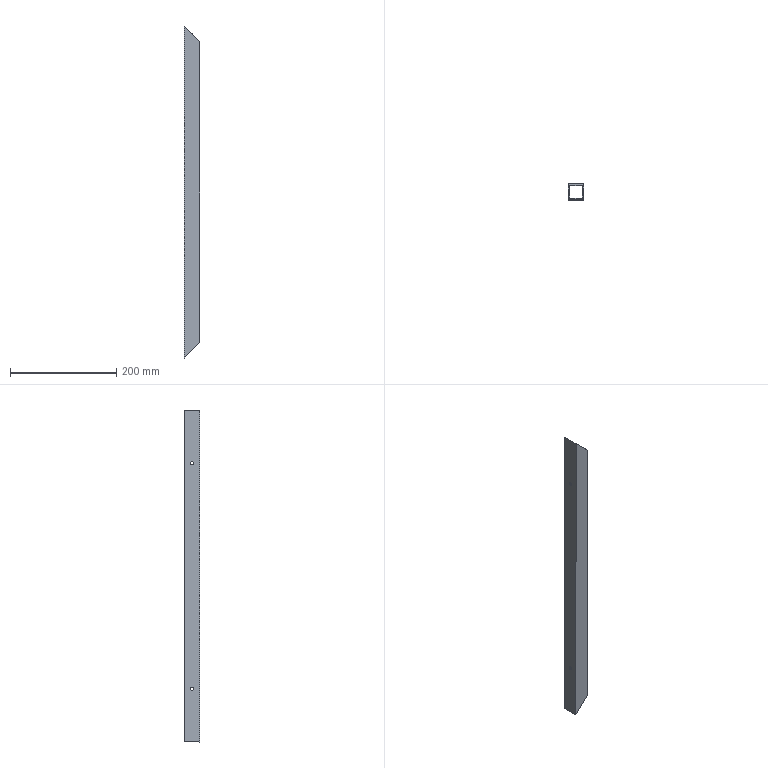Part | SolidWorks | features Cut 2, Extrusion 1, ICE 1 | 1 solid | 18 faces | box 30 x 30 x 625.685 mm | volume 192663 mm3 | plane 10 | cylinder 8 | commonest cylinder face diameters 6 x8
STEP:
#1=CARTESIAN_POINT('',(-39.774,34.622,225.979));
#2=VERTEX_POINT('',#1);
#3=CARTESIAN_POINT('',(-39.774,28.622,225.979));
#4=VERTEX_POINT('',#3);
#5=CARTESIAN_POINT('',(-39.774,31.622,225.979));
#6=DIRECTION('',(-1.,0.,0.));
#7=DIRECTION('',(0.,0.,1.));
#8=AXIS2_PLACEMENT_3D('',#5,#6,#7);
#9=CIRCLE('',#8,3.);
#10=EDGE_CURVE('',#2,#4,#9,.T.);
#11=ORIENTED_EDGE('',*,*,#10,.F.);
#12=CARTESIAN_POINT('',(-42.774,34.622,225.979));
#13=VERTEX_POINT('',#12);
#14=CARTESIAN_POINT('',(-12.774,34.622,225.979));
#15=DIRECTION('',(-1.,0.,0.));
#16=VECTOR('',#15,1000.);
#17=LINE('',#14,#16);
#18=EDGE_CURVE('',#2,#13,#17,.T.);
#19=ORIENTED_EDGE('',*,*,#18,.T.);
#20=CARTESIAN_POINT('',(-42.774,28.622,225.979));
#21=VERTEX_POINT('',#20);
#22=CARTESIAN_POINT('',(-42.774,31.622,225.979));
#23=DIRECTION('',(1.,0.,0.));
#24=DIRECTION('',(0.,0.,-1.));
#25=AXIS2_PLACEMENT_3D('',#22,#23,#24);
#26=CIRCLE('',#25,3.);
#27=EDGE_CURVE('',#21,#13,#26,.T.);
#28=ORIENTED_EDGE('',*,*,#27,.F.);
#29=CARTESIAN_POINT('',(-12.774,28.622,225.979));
#30=DIRECTION('',(-1.,0.,0.));
#31=VECTOR('',#30,1000.);
#32=LINE('',#29,#31);
#33=EDGE_CURVE('',#4,#21,#32,.T.);
#34=ORIENTED_EDGE('',*,*,#33,.F.);
#35=EDGE_LOOP('',(#11,#19,#28,#34));
#36=FACE_OUTER_BOUND('',#35,.T.);
#37=CARTESIAN_POINT('',(-12.774,31.622,225.979));
#38=DIRECTION('',(-1.,0.,0.));
#39=DIRECTION('',(0.,-1.,0.));
#40=AXIS2_PLACEMENT_3D('',#37,#38,#39);
#41=CYLINDRICAL_SURFACE('',#40,3.);
#42=ADVANCED_FACE('',(#36),#41,.F.);
#43=CARTESIAN_POINT('',(-39.774,34.622,651.665));
#44=VERTEX_POINT('',#43);
#45=CARTESIAN_POINT('',(-39.774,28.622,651.665));
#46=VERTEX_POINT('',#45);
#47=CARTESIAN_POINT('',(-39.774,31.622,651.665));
#48=DIRECTION('',(-1.,0.,0.));
#49=DIRECTION('',(0.,0.,1.));
#50=AXIS2_PLACEMENT_3D('',#47,#48,#49);
#51=CIRCLE('',#50,3.);
#52=EDGE_CURVE('',#44,#46,#51,.T.);
#53=ORIENTED_EDGE('',*,*,#52,.F.);
#54=CARTESIAN_POINT('',(-42.774,34.622,651.665));
#55=VERTEX_POINT('',#54);
#56=CARTESIAN_POINT('',(-12.774,34.622,651.665));
#57=DIRECTION('',(-1.,0.,0.));
#58=VECTOR('',#57,1000.);
#59=LINE('',#56,#58);
#60=EDGE_CURVE('',#44,#55,#59,.T.);
#61=ORIENTED_EDGE('',*,*,#60,.T.);
#62=CARTESIAN_POINT('',(-42.774,28.622,651.665));
#63=VERTEX_POINT('',#62);
#64=CARTESIAN_POINT('',(-42.774,31.622,651.665));
#65=DIRECTION('',(1.,0.,0.));
#66=DIRECTION('',(0.,0.,-1.));
#67=AXIS2_PLACEMENT_3D('',#64,#65,#66);
#68=CIRCLE('',#67,3.);
#69=EDGE_CURVE('',#63,#55,#68,.T.);
#70=ORIENTED_EDGE('',*,*,#69,.F.);
#71=CARTESIAN_POINT('',(-12.774,28.622,651.665));
#72=DIRECTION('',(-1.,0.,0.));
#73=VECTOR('',#72,1000.);
#74=LINE('',#71,#73);
#75=EDGE_CURVE('',#46,#63,#74,.T.);
#76=ORIENTED_EDGE('',*,*,#75,.F.);
#77=EDGE_LOOP('',(#53,#61,#70,#76));
#78=FACE_OUTER_BOUND('',#77,.T.);
#79=CARTESIAN_POINT('',(-12.774,31.622,651.665));
#80=DIRECTION('',(-1.,0.,0.));
#81=DIRECTION('',(0.,-1.,0.));
#82=AXIS2_PLACEMENT_3D('',#79,#80,#81);
#83=CYLINDRICAL_SURFACE('',#82,3.);
#84=ADVANCED_FACE('',(#78),#83,.F.);
#85=CARTESIAN_POINT('',(-12.774,34.622,225.979));
#86=VERTEX_POINT('',#85);
#87=CARTESIAN_POINT('',(-12.774,28.622,225.979));
#88=VERTEX_POINT('',#87);
#89=CARTESIAN_POINT('',(-12.774,31.622,225.979));
#90=DIRECTION('',(-1.,0.,0.));
#91=DIRECTION('',(0.,-1.,0.));
#92=AXIS2_PLACEMENT_3D('',#89,#90,#91);
#93=CIRCLE('',#92,3.);
#94=EDGE_CURVE('',#86,#88,#93,.T.);
#95=ORIENTED_EDGE('',*,*,#94,.F.);
#96=CARTESIAN_POINT('',(-15.774,34.622,225.979));
#97=VERTEX_POINT('',#96);
#98=CARTESIAN_POINT('',(-12.774,34.622,225.979));
#99=DIRECTION('',(-1.,0.,0.));
#100=VECTOR('',#99,1000.);
#101=LINE('',#98,#100);
#102=EDGE_CURVE('',#86,#97,#101,.T.);
#103=ORIENTED_EDGE('',*,*,#102,.T.);
#104=CARTESIAN_POINT('',(-15.774,28.622,225.979));
#105=VERTEX_POINT('',#104);
#106=CARTESIAN_POINT('',(-15.774,31.622,225.979));
#107=DIRECTION('',(1.,0.,0.));
#108=DIRECTION('',(0.,1.,0.));
#109=AXIS2_PLACEMENT_3D('',#106,#107,#108);
#110=CIRCLE('',#109,3.);
#111=EDGE_CURVE('',#105,#97,#110,.T.);
#112=ORIENTED_EDGE('',*,*,#111,.F.);
#113=CARTESIAN_POINT('',(-12.774,28.622,225.979));
#114=DIRECTION('',(-1.,0.,0.));
#115=VECTOR('',#114,1000.);
#116=LINE('',#113,#115);
#117=EDGE_CURVE('',#88,#105,#116,.T.);
#118=ORIENTED_EDGE('',*,*,#117,.F.);
#119=EDGE_LOOP('',(#95,#103,#112,#118));
#120=FACE_OUTER_BOUND('',#119,.T.);
#121=CARTESIAN_POINT('',(-12.774,31.622,225.979));
#122=DIRECTION('',(-1.,0.,0.));
#123=DIRECTION('',(0.,-1.,0.));
#124=AXIS2_PLACEMENT_3D('',#121,#122,#123);
#125=CYLINDRICAL_SURFACE('',#124,3.);
#126=ADVANCED_FACE('',(#120),#125,.F.);
#127=CARTESIAN_POINT('',(-12.774,34.622,651.665));
#128=VERTEX_POINT('',#127);
#129=CARTESIAN_POINT('',(-12.774,28.622,651.665));
#130=VERTEX_POINT('',#129);
#131=CARTESIAN_POINT('',(-12.774,31.622,651.665));
#132=DIRECTION('',(-1.,0.,0.));
#133=DIRECTION('',(0.,-1.,0.));
#134=AXIS2_PLACEMENT_3D('',#131,#132,#133);
#135=CIRCLE('',#134,3.);
#136=EDGE_CURVE('',#128,#130,#135,.T.);
#137=ORIENTED_EDGE('',*,*,#136,.F.);
#138=CARTESIAN_POINT('',(-15.774,34.622,651.665));
#139=VERTEX_POINT('',#138);
#140=CARTESIAN_POINT('',(-12.774,34.622,651.665));
#141=DIRECTION('',(-1.,0.,0.));
#142=VECTOR('',#141,1000.);
#143=LINE('',#140,#142);
#144=EDGE_CURVE('',#128,#139,#143,.T.);
#145=ORIENTED_EDGE('',*,*,#144,.T.);
#146=CARTESIAN_POINT('',(-15.774,28.622,651.665));
#147=VERTEX_POINT('',#146);
#148=CARTESIAN_POINT('',(-15.774,31.622,651.665));
#149=DIRECTION('',(1.,0.,0.));
#150=DIRECTION('',(0.,1.,0.));
#151=AXIS2_PLACEMENT_3D('',#148,#149,#150);
#152=CIRCLE('',#151,3.);
#153=EDGE_CURVE('',#147,#139,#152,.T.);
#154=ORIENTED_EDGE('',*,*,#153,.F.);
#155=CARTESIAN_POINT('',(-12.774,28.622,651.665));
#156=DIRECTION('',(-1.,0.,0.));
#157=VECTOR('',#156,1000.);
#158=LINE('',#155,#157);
#159=EDGE_CURVE('',#130,#147,#158,.T.);
#160=ORIENTED_EDGE('',*,*,#159,.F.);
#161=EDGE_LOOP('',(#137,#145,#154,#160));
#162=FACE_OUTER_BOUND('',#161,.T.);
#163=CARTESIAN_POINT('',(-12.774,31.622,651.665));
#164=DIRECTION('',(-1.,0.,0.));
#165=DIRECTION('',(0.,-1.,0.));
#166=AXIS2_PLACEMENT_3D('',#163,#164,#165);
#167=CYLINDRICAL_SURFACE('',#166,3.);
#168=ADVANCED_FACE('',(#162),#167,.F.);
#169=CARTESIAN_POINT('',(-39.774,19.622,128.979));
#170=VERTEX_POINT('',#169);
#171=CARTESIAN_POINT('',(-39.774,19.622,748.665));
#172=VERTEX_POINT('',#171);
#173=CARTESIAN_POINT('',(-39.774,19.622,0.));
#174=DIRECTION('',(0.,0.,1.));
#175=VECTOR('',#174,1000.);
#176=LINE('',#173,#175);
#177=EDGE_CURVE('',#170,#172,#176,.T.);
#178=ORIENTED_EDGE('',*,*,#177,.T.);
#179=CARTESIAN_POINT('',(-15.774,19.622,724.665));
#180=VERTEX_POINT('',#179);
#181=CARTESIAN_POINT('',(346.559,19.622,362.332));
#182=DIRECTION('',(0.7071,0.,-0.7071));
#183=VECTOR('',#182,1000.);
#184=LINE('',#181,#183);
#185=EDGE_CURVE('',#172,#180,#184,.T.);
#186=ORIENTED_EDGE('',*,*,#185,.T.);
#187=CARTESIAN_POINT('',(-15.774,19.622,152.979));
#188=VERTEX_POINT('',#187);
#189=CARTESIAN_POINT('',(-15.774,19.622,0.));
#190=DIRECTION('',(0.,0.,1.));
#191=VECTOR('',#190,1000.);
#192=LINE('',#189,#191);
#193=EDGE_CURVE('',#188,#180,#192,.T.);
#194=ORIENTED_EDGE('',*,*,#193,.F.);
#195=CARTESIAN_POINT('',(-92.263,19.622,76.49));
#196=DIRECTION('',(-0.7071,0.,-0.7071));
#197=VECTOR('',#196,1000.);
#198=LINE('',#195,#197);
#199=EDGE_CURVE('',#188,#170,#198,.T.);
#200=ORIENTED_EDGE('',*,*,#199,.T.);
#201=EDGE_LOOP('',(#178,#186,#194,#200));
#202=FACE_OUTER_BOUND('',#201,.T.);
#203=CARTESIAN_POINT('',(-15.774,19.622,0.));
#204=DIRECTION('',(0.,-1.,0.));
#205=DIRECTION('',(1.,0.,0.));
#206=AXIS2_PLACEMENT_3D('',#203,#204,#205);
#207=PLANE('',#206);
#208=ADVANCED_FACE('',(#202),#207,.F.);
#209=ORIENTED_EDGE('',*,*,#111,.T.);
#210=CARTESIAN_POINT('',(-15.774,31.622,225.979));
#211=DIRECTION('',(1.,0.,0.));
#212=DIRECTION('',(0.,1.,0.));
#213=AXIS2_PLACEMENT_3D('',#210,#211,#212);
#214=CIRCLE('',#213,3.);
#215=EDGE_CURVE('',#97,#105,#214,.T.);
#216=ORIENTED_EDGE('',*,*,#215,.T.);
#217=EDGE_LOOP('',(#209,#216));
#218=FACE_BOUND('',#217,.T.);
#219=ORIENTED_EDGE('',*,*,#153,.T.);
#220=CARTESIAN_POINT('',(-15.774,31.622,651.665));
#221=DIRECTION('',(1.,0.,0.));
#222=DIRECTION('',(0.,1.,0.));
#223=AXIS2_PLACEMENT_3D('',#220,#221,#222);
#224=CIRCLE('',#223,3.);
#225=EDGE_CURVE('',#139,#147,#224,.T.);
#226=ORIENTED_EDGE('',*,*,#225,.T.);
#227=EDGE_LOOP('',(#219,#226));
#228=FACE_BOUND('',#227,.T.);
#229=ORIENTED_EDGE('',*,*,#193,.T.);
#230=CARTESIAN_POINT('',(-15.774,43.622,724.665));
#231=VERTEX_POINT('',#230);
#232=CARTESIAN_POINT('',(-15.774,43.622,724.665));
#233=DIRECTION('',(0.,1.,0.));
#234=VECTOR('',#233,1000.);
#235=LINE('',#232,#234);
#236=EDGE_CURVE('',#180,#231,#235,.T.);
#237=ORIENTED_EDGE('',*,*,#236,.T.);
#238=CARTESIAN_POINT('',(-15.774,43.622,152.979));
#239=VERTEX_POINT('',#238);
#240=CARTESIAN_POINT('',(-15.774,43.622,0.));
#241=DIRECTION('',(0.,0.,1.));
#242=VECTOR('',#241,1000.);
#243=LINE('',#240,#242);
#244=EDGE_CURVE('',#239,#231,#243,.T.);
#245=ORIENTED_EDGE('',*,*,#244,.F.);
#246=CARTESIAN_POINT('',(-15.774,43.622,152.979));
#247=DIRECTION('',(0.,-1.,0.));
#248=VECTOR('',#247,1000.);
#249=LINE('',#246,#248);
#250=EDGE_CURVE('',#239,#188,#249,.T.);
#251=ORIENTED_EDGE('',*,*,#250,.T.);
#252=EDGE_LOOP('',(#229,#237,#245,#251));
#253=FACE_OUTER_BOUND('',#252,.T.);
#254=CARTESIAN_POINT('',(-15.774,43.622,0.));
#255=DIRECTION('',(1.,0.,0.));
#256=DIRECTION('',(0.,1.,0.));
#257=AXIS2_PLACEMENT_3D('',#254,#255,#256);
#258=PLANE('',#257);
#259=ADVANCED_FACE('',(#218,#228,#253),#258,.F.);
#260=ORIENTED_EDGE('',*,*,#244,.T.);
#261=CARTESIAN_POINT('',(-39.774,43.622,748.665));
#262=VERTEX_POINT('',#261);
#263=CARTESIAN_POINT('',(334.559,43.622,374.332));
#264=DIRECTION('',(-0.7071,0.,0.7071));
#265=VECTOR('',#264,1000.);
#266=LINE('',#263,#265);
#267=EDGE_CURVE('',#231,#262,#266,.T.);
#268=ORIENTED_EDGE('',*,*,#267,.T.);
#269=CARTESIAN_POINT('',(-39.774,43.622,128.979));
#270=VERTEX_POINT('',#269);
#271=CARTESIAN_POINT('',(-39.774,43.622,0.));
#272=DIRECTION('',(0.,0.,1.));
#273=VECTOR('',#272,1000.);
#274=LINE('',#271,#273);
#275=EDGE_CURVE('',#270,#262,#274,.T.);
#276=ORIENTED_EDGE('',*,*,#275,.F.);
#277=CARTESIAN_POINT('',(-104.263,43.622,64.49));
#278=DIRECTION('',(0.7071,0.,0.7071));
#279=VECTOR('',#278,1000.);
#280=LINE('',#277,#279);
#281=EDGE_CURVE('',#270,#239,#280,.T.);
#282=ORIENTED_EDGE('',*,*,#281,.T.);
#283=EDGE_LOOP('',(#260,#268,#276,#282));
#284=FACE_OUTER_BOUND('',#283,.T.);
#285=CARTESIAN_POINT('',(-39.774,43.622,0.));
#286=DIRECTION('',(0.,1.,0.));
#287=DIRECTION('',(0.,0.,1.));
#288=AXIS2_PLACEMENT_3D('',#285,#286,#287);
#289=PLANE('',#288);
#290=ADVANCED_FACE('',(#284),#289,.F.);
#291=CARTESIAN_POINT('',(-39.774,31.622,225.979));
#292=DIRECTION('',(-1.,0.,0.));
#293=DIRECTION('',(0.,0.,1.));
#294=AXIS2_PLACEMENT_3D('',#291,#292,#293);
#295=CIRCLE('',#294,3.);
#296=EDGE_CURVE('',#4,#2,#295,.T.);
#297=ORIENTED_EDGE('',*,*,#296,.T.);
#298=ORIENTED_EDGE('',*,*,#10,.T.);
#299=EDGE_LOOP('',(#297,#298));
#300=FACE_BOUND('',#299,.T.);
#301=CARTESIAN_POINT('',(-39.774,31.622,651.665));
#302=DIRECTION('',(-1.,0.,0.));
#303=DIRECTION('',(0.,0.,1.));
#304=AXIS2_PLACEMENT_3D('',#301,#302,#303);
#305=CIRCLE('',#304,3.);
#306=EDGE_CURVE('',#46,#44,#305,.T.);
#307=ORIENTED_EDGE('',*,*,#306,.T.);
#308=ORIENTED_EDGE('',*,*,#52,.T.);
#309=EDGE_LOOP('',(#307,#308));
#310=FACE_BOUND('',#309,.T.);
#311=ORIENTED_EDGE('',*,*,#275,.T.);
#312=CARTESIAN_POINT('',(-39.774,19.622,748.665));
#313=DIRECTION('',(0.,-1.,0.));
#314=VECTOR('',#313,1000.);
#315=LINE('',#312,#314);
#316=EDGE_CURVE('',#262,#172,#315,.T.);
#317=ORIENTED_EDGE('',*,*,#316,.T.);
#318=ORIENTED_EDGE('',*,*,#177,.F.);
#319=CARTESIAN_POINT('',(-39.774,19.622,128.979));
#320=DIRECTION('',(0.,1.,0.));
#321=VECTOR('',#320,1000.);
#322=LINE('',#319,#321);
#323=EDGE_CURVE('',#170,#270,#322,.T.);
#324=ORIENTED_EDGE('',*,*,#323,.T.);
#325=EDGE_LOOP('',(#311,#317,#318,#324));
#326=FACE_OUTER_BOUND('',#325,.T.);
#327=CARTESIAN_POINT('',(-39.774,19.622,0.));
#328=DIRECTION('',(-1.,0.,0.));
#329=DIRECTION('',(0.,0.,1.));
#330=AXIS2_PLACEMENT_3D('',#327,#328,#329);
#331=PLANE('',#330);
#332=ADVANCED_FACE('',(#300,#310,#326),#331,.F.);
#333=CARTESIAN_POINT('',(-12.774,16.622,155.979));
#334=VERTEX_POINT('',#333);
#335=CARTESIAN_POINT('',(-42.774,16.622,125.979));
#336=VERTEX_POINT('',#335);
#337=CARTESIAN_POINT('',(-12.774,16.622,155.979));
#338=DIRECTION('',(-0.7071,0.,-0.7071));
#339=VECTOR('',#338,1000.);
#340=LINE('',#337,#339);
#341=EDGE_CURVE('',#334,#336,#340,.T.);
#342=ORIENTED_EDGE('',*,*,#341,.T.);
#343=CARTESIAN_POINT('',(-42.774,46.622,125.979));
#344=VERTEX_POINT('',#343);
#345=CARTESIAN_POINT('',(-42.774,46.622,125.979));
#346=DIRECTION('',(0.,-1.,0.));
#347=VECTOR('',#346,1000.);
#348=LINE('',#345,#347);
#349=EDGE_CURVE('',#344,#336,#348,.T.);
#350=ORIENTED_EDGE('',*,*,#349,.F.);
#351=CARTESIAN_POINT('',(-12.774,46.622,155.979));
#352=VERTEX_POINT('',#351);
#353=CARTESIAN_POINT('',(-12.774,46.622,155.979));
#354=DIRECTION('',(-0.7071,0.,-0.7071));
#355=VECTOR('',#354,1000.);
#356=LINE('',#353,#355);
#357=EDGE_CURVE('',#352,#344,#356,.T.);
#358=ORIENTED_EDGE('',*,*,#357,.F.);
#359=CARTESIAN_POINT('',(-12.774,46.622,155.979));
#360=DIRECTION('',(0.,-1.,0.));
#361=VECTOR('',#360,1000.);
#362=LINE('',#359,#361);
#363=EDGE_CURVE('',#352,#334,#362,.T.);
#364=ORIENTED_EDGE('',*,*,#363,.T.);
#365=EDGE_LOOP('',(#342,#350,#358,#364));
#366=FACE_OUTER_BOUND('',#365,.T.);
#367=ORIENTED_EDGE('',*,*,#199,.F.);
#368=ORIENTED_EDGE('',*,*,#250,.F.);
#369=ORIENTED_EDGE('',*,*,#281,.F.);
#370=ORIENTED_EDGE('',*,*,#323,.F.);
#371=EDGE_LOOP('',(#367,#368,#369,#370));
#372=FACE_BOUND('',#371,.T.);
#373=CARTESIAN_POINT('',(-12.774,46.622,155.979));
#374=DIRECTION('',(-0.7071,0.,0.7071));
#375=DIRECTION('',(0.7071,0.,0.7071));
#376=AXIS2_PLACEMENT_3D('',#373,#374,#375);
#377=PLANE('',#376);
#378=ADVANCED_FACE('',(#366,#372),#377,.F.);
#379=CARTESIAN_POINT('',(-42.774,16.622,751.665));
#380=VERTEX_POINT('',#379);
#381=CARTESIAN_POINT('',(-12.774,16.622,721.665));
#382=VERTEX_POINT('',#381);
#383=CARTESIAN_POINT('',(-12.774,16.622,721.665));
#384=DIRECTION('',(0.7071,0.,-0.7071));
#385=VECTOR('',#384,1000.);
#386=LINE('',#383,#385);
#387=EDGE_CURVE('',#380,#382,#386,.T.);
#388=ORIENTED_EDGE('',*,*,#387,.T.);
#389=CARTESIAN_POINT('',(-12.774,46.622,721.665));
#390=VERTEX_POINT('',#389);
#391=CARTESIAN_POINT('',(-12.774,46.622,721.665));
#392=DIRECTION('',(0.,-1.,0.));
#393=VECTOR('',#392,1000.);
#394=LINE('',#391,#393);
#395=EDGE_CURVE('',#390,#382,#394,.T.);
#396=ORIENTED_EDGE('',*,*,#395,.F.);
#397=CARTESIAN_POINT('',(-42.774,46.622,751.665));
#398=VERTEX_POINT('',#397);
#399=CARTESIAN_POINT('',(-12.774,46.622,721.665));
#400=DIRECTION('',(0.7071,0.,-0.7071));
#401=VECTOR('',#400,1000.);
#402=LINE('',#399,#401);
#403=EDGE_CURVE('',#398,#390,#402,.T.);
#404=ORIENTED_EDGE('',*,*,#403,.F.);
#405=CARTESIAN_POINT('',(-42.774,46.622,751.665));
#406=DIRECTION('',(0.,-1.,0.));
#407=VECTOR('',#406,1000.);
#408=LINE('',#405,#407);
#409=EDGE_CURVE('',#398,#380,#408,.T.);
#410=ORIENTED_EDGE('',*,*,#409,.T.);
#411=EDGE_LOOP('',(#388,#396,#404,#410));
#412=FACE_OUTER_BOUND('',#411,.T.);
#413=ORIENTED_EDGE('',*,*,#267,.F.);
#414=ORIENTED_EDGE('',*,*,#236,.F.);
#415=ORIENTED_EDGE('',*,*,#185,.F.);
#416=ORIENTED_EDGE('',*,*,#316,.F.);
#417=EDGE_LOOP('',(#413,#414,#415,#416));
#418=FACE_BOUND('',#417,.T.);
#419=CARTESIAN_POINT('',(-12.774,46.622,721.665));
#420=DIRECTION('',(-0.7071,0.,-0.7071));
#421=DIRECTION('',(-0.7071,0.,0.7071));
#422=AXIS2_PLACEMENT_3D('',#419,#420,#421);
#423=PLANE('',#422);
#424=ADVANCED_FACE('',(#412,#418),#423,.F.);
#425=ORIENTED_EDGE('',*,*,#27,.T.);
#426=CARTESIAN_POINT('',(-42.774,31.622,225.979));
#427=DIRECTION('',(1.,0.,0.));
#428=DIRECTION('',(0.,0.,-1.));
#429=AXIS2_PLACEMENT_3D('',#426,#427,#428);
#430=CIRCLE('',#429,3.);
#431=EDGE_CURVE('',#13,#21,#430,.T.);
#432=ORIENTED_EDGE('',*,*,#431,.T.);
#433=EDGE_LOOP('',(#425,#432));
#434=FACE_BOUND('',#433,.T.);
#435=ORIENTED_EDGE('',*,*,#69,.T.);
#436=CARTESIAN_POINT('',(-42.774,31.622,651.665));
#437=DIRECTION('',(1.,0.,0.));
#438=DIRECTION('',(0.,0.,-1.));
#439=AXIS2_PLACEMENT_3D('',#436,#437,#438);
#440=CIRCLE('',#439,3.);
#441=EDGE_CURVE('',#55,#63,#440,.T.);
#442=ORIENTED_EDGE('',*,*,#441,.T.);
#443=EDGE_LOOP('',(#435,#442));
#444=FACE_BOUND('',#443,.T.);
#445=CARTESIAN_POINT('',(-42.774,16.622,800.));
#446=DIRECTION('',(0.,0.,-1.));
#447=VECTOR('',#446,1000.);
#448=LINE('',#445,#447);
#449=EDGE_CURVE('',#380,#336,#448,.T.);
#450=ORIENTED_EDGE('',*,*,#449,.F.);
#451=ORIENTED_EDGE('',*,*,#409,.F.);
#452=CARTESIAN_POINT('',(-42.774,46.622,800.));
#453=DIRECTION('',(0.,0.,-1.));
#454=VECTOR('',#453,1000.);
#455=LINE('',#452,#454);
#456=EDGE_CURVE('',#398,#344,#455,.T.);
#457=ORIENTED_EDGE('',*,*,#456,.T.);
#458=ORIENTED_EDGE('',*,*,#349,.T.);
#459=EDGE_LOOP('',(#450,#451,#457,#458));
#460=FACE_OUTER_BOUND('',#459,.T.);
#461=CARTESIAN_POINT('',(-42.774,16.622,800.));
#462=DIRECTION('',(1.,0.,0.));
#463=DIRECTION('',(0.,0.,-1.));
#464=AXIS2_PLACEMENT_3D('',#461,#462,#463);
#465=PLANE('',#464);
#466=ADVANCED_FACE('',(#434,#444,#460),#465,.F.);
#467=CARTESIAN_POINT('',(-12.774,16.622,800.));
#468=DIRECTION('',(0.,0.,-1.));
#469=VECTOR('',#468,1000.);
#470=LINE('',#467,#469);
#471=EDGE_CURVE('',#382,#334,#470,.T.);
#472=ORIENTED_EDGE('',*,*,#471,.F.);
#473=ORIENTED_EDGE('',*,*,#387,.F.);
#474=ORIENTED_EDGE('',*,*,#449,.T.);
#475=ORIENTED_EDGE('',*,*,#341,.F.);
#476=EDGE_LOOP('',(#472,#473,#474,#475));
#477=FACE_OUTER_BOUND('',#476,.T.);
#478=CARTESIAN_POINT('',(-12.774,16.622,800.));
#479=DIRECTION('',(0.,1.,0.));
#480=DIRECTION('',(0.,0.,1.));
#481=AXIS2_PLACEMENT_3D('',#478,#479,#480);
#482=PLANE('',#481);
#483=ADVANCED_FACE('',(#477),#482,.F.);
#484=CARTESIAN_POINT('',(-12.774,31.622,225.979));
#485=DIRECTION('',(-1.,0.,0.));
#486=DIRECTION('',(0.,-1.,0.));
#487=AXIS2_PLACEMENT_3D('',#484,#485,#486);
#488=CIRCLE('',#487,3.);
#489=EDGE_CURVE('',#88,#86,#488,.T.);
#490=ORIENTED_EDGE('',*,*,#489,.T.);
#491=ORIENTED_EDGE('',*,*,#94,.T.);
#492=EDGE_LOOP('',(#490,#491));
#493=FACE_BOUND('',#492,.T.);
#494=CARTESIAN_POINT('',(-12.774,31.622,651.665));
#495=DIRECTION('',(-1.,0.,0.));
#496=DIRECTION('',(0.,-1.,0.));
#497=AXIS2_PLACEMENT_3D('',#494,#495,#496);
#498=CIRCLE('',#497,3.);
#499=EDGE_CURVE('',#130,#128,#498,.T.);
#500=ORIENTED_EDGE('',*,*,#499,.T.);
#501=ORIENTED_EDGE('',*,*,#136,.T.);
#502=EDGE_LOOP('',(#500,#501));
#503=FACE_BOUND('',#502,.T.);
#504=CARTESIAN_POINT('',(-12.774,46.622,800.));
#505=DIRECTION('',(0.,0.,-1.));
#506=VECTOR('',#505,1000.);
#507=LINE('',#504,#506);
#508=EDGE_CURVE('',#390,#352,#507,.T.);
#509=ORIENTED_EDGE('',*,*,#508,.F.);
#510=ORIENTED_EDGE('',*,*,#395,.T.);
#511=ORIENTED_EDGE('',*,*,#471,.T.);
#512=ORIENTED_EDGE('',*,*,#363,.F.);
#513=EDGE_LOOP('',(#509,#510,#511,#512));
#514=FACE_OUTER_BOUND('',#513,.T.);
#515=CARTESIAN_POINT('',(-12.774,46.622,800.));
#516=DIRECTION('',(-1.,0.,0.));
#517=DIRECTION('',(0.,0.,1.));
#518=AXIS2_PLACEMENT_3D('',#515,#516,#517);
#519=PLANE('',#518);
#520=ADVANCED_FACE('',(#493,#503,#514),#519,.F.);
#521=ORIENTED_EDGE('',*,*,#456,.F.);
#522=ORIENTED_EDGE('',*,*,#403,.T.);
#523=ORIENTED_EDGE('',*,*,#508,.T.);
#524=ORIENTED_EDGE('',*,*,#357,.T.);
#525=EDGE_LOOP('',(#521,#522,#523,#524));
#526=FACE_OUTER_BOUND('',#525,.T.);
#527=CARTESIAN_POINT('',(-42.774,46.622,800.));
#528=DIRECTION('',(0.,-1.,0.));
#529=DIRECTION('',(0.,0.,-1.));
#530=AXIS2_PLACEMENT_3D('',#527,#528,#529);
#531=PLANE('',#530);
#532=ADVANCED_FACE('',(#526),#531,.F.);
#533=ORIENTED_EDGE('',*,*,#144,.F.);
#534=ORIENTED_EDGE('',*,*,#499,.F.);
#535=ORIENTED_EDGE('',*,*,#159,.T.);
#536=ORIENTED_EDGE('',*,*,#225,.F.);
#537=EDGE_LOOP('',(#533,#534,#535,#536));
#538=FACE_OUTER_BOUND('',#537,.T.);
#539=CARTESIAN_POINT('',(-12.774,31.622,651.665));
#540=DIRECTION('',(-1.,0.,0.));
#541=DIRECTION('',(0.,-1.,0.));
#542=AXIS2_PLACEMENT_3D('',#539,#540,#541);
#543=CYLINDRICAL_SURFACE('',#542,3.);
#544=ADVANCED_FACE('',(#538),#543,.F.);
#545=ORIENTED_EDGE('',*,*,#102,.F.);
#546=ORIENTED_EDGE('',*,*,#489,.F.);
#547=ORIENTED_EDGE('',*,*,#117,.T.);
#548=ORIENTED_EDGE('',*,*,#215,.F.);
#549=EDGE_LOOP('',(#545,#546,#547,#548));
#550=FACE_OUTER_BOUND('',#549,.T.);
#551=CARTESIAN_POINT('',(-12.774,31.622,225.979));
#552=DIRECTION('',(-1.,0.,0.));
#553=DIRECTION('',(0.,-1.,0.));
#554=AXIS2_PLACEMENT_3D('',#551,#552,#553);
#555=CYLINDRICAL_SURFACE('',#554,3.);
#556=ADVANCED_FACE('',(#550),#555,.F.);
#557=ORIENTED_EDGE('',*,*,#60,.F.);
#558=ORIENTED_EDGE('',*,*,#306,.F.);
#559=ORIENTED_EDGE('',*,*,#75,.T.);
#560=ORIENTED_EDGE('',*,*,#441,.F.);
#561=EDGE_LOOP('',(#557,#558,#559,#560));
#562=FACE_OUTER_BOUND('',#561,.T.);
#563=CARTESIAN_POINT('',(-12.774,31.622,651.665));
#564=DIRECTION('',(-1.,0.,0.));
#565=DIRECTION('',(0.,-1.,0.));
#566=AXIS2_PLACEMENT_3D('',#563,#564,#565);
#567=CYLINDRICAL_SURFACE('',#566,3.);
#568=ADVANCED_FACE('',(#562),#567,.F.);
#569=ORIENTED_EDGE('',*,*,#18,.F.);
#570=ORIENTED_EDGE('',*,*,#296,.F.);
#571=ORIENTED_EDGE('',*,*,#33,.T.);
#572=ORIENTED_EDGE('',*,*,#431,.F.);
#573=EDGE_LOOP('',(#569,#570,#571,#572));
#574=FACE_OUTER_BOUND('',#573,.T.);
#575=CARTESIAN_POINT('',(-12.774,31.622,225.979));
#576=DIRECTION('',(-1.,0.,0.));
#577=DIRECTION('',(0.,-1.,0.));
#578=AXIS2_PLACEMENT_3D('',#575,#576,#577);
#579=CYLINDRICAL_SURFACE('',#578,3.);
#580=ADVANCED_FACE('',(#574),#579,.F.);
#581=CLOSED_SHELL('',(#42,#84,#126,#168,#208,#259,#290,#332,#378,#424,#466,#483,#520,#532,#544,#556,#568,#580));
#582=MANIFOLD_SOLID_BREP('',#581);
#583=CARTESIAN_POINT('',(0.,0.,0.));
#584=DIRECTION('',(0.,0.,1.));
#585=DIRECTION('',(1.,0.,0.));
#586=AXIS2_PLACEMENT_3D('',#583,#584,#585);
#587=(LENGTH_UNIT()NAMED_UNIT(*)SI_UNIT(.MILLI.,.METRE.));
#588=UNCERTAINTY_MEASURE_WITH_UNIT(LENGTH_MEASURE(0.00001),#587,'','');
#589=(NAMED_UNIT(*)PLANE_ANGLE_UNIT()SI_UNIT($,.RADIAN.));
#590=(NAMED_UNIT(*)SI_UNIT($,.STERADIAN.)SOLID_ANGLE_UNIT());
#591=(GEOMETRIC_REPRESENTATION_CONTEXT(3)GLOBAL_UNCERTAINTY_ASSIGNED_CONTEXT((#588))GLOBAL_UNIT_ASSIGNED_CONTEXT((#587,#589,#590))REPRESENTATION_CONTEXT('',''));
#592=ADVANCED_BREP_SHAPE_REPRESENTATION('',(#582,#586),#591);